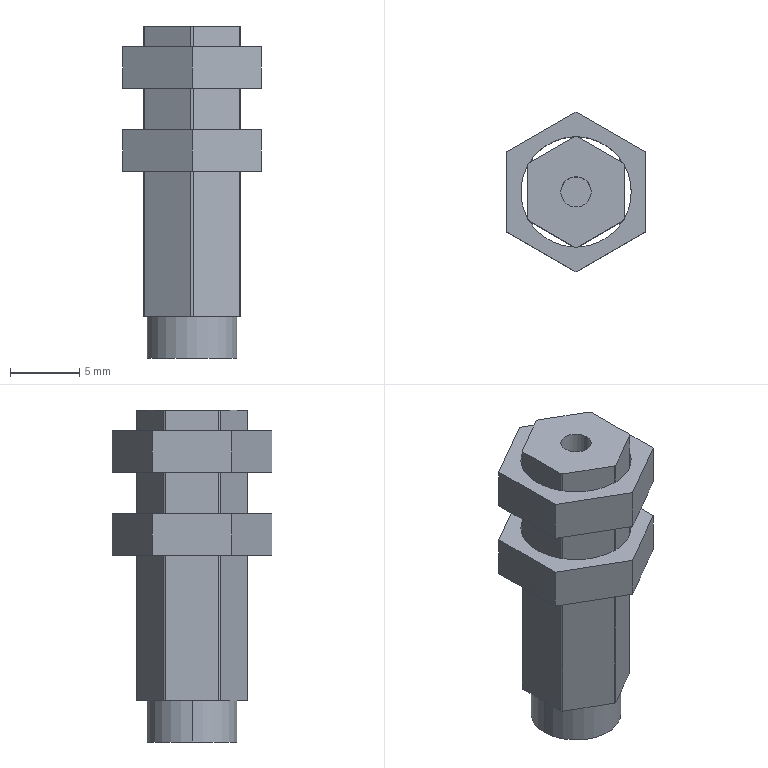Part | STEP file | body_A_CJPS4_10_B_0_ | 1 solid | 65 faces | box 10 x 11.547 x 24 mm | volume 1164 mm3 | cylinder 38 | plane 27 | commonest cylinder face diameters 8 x18 7.98 x14 0.4 x2 2.2 x2 6.5 x2